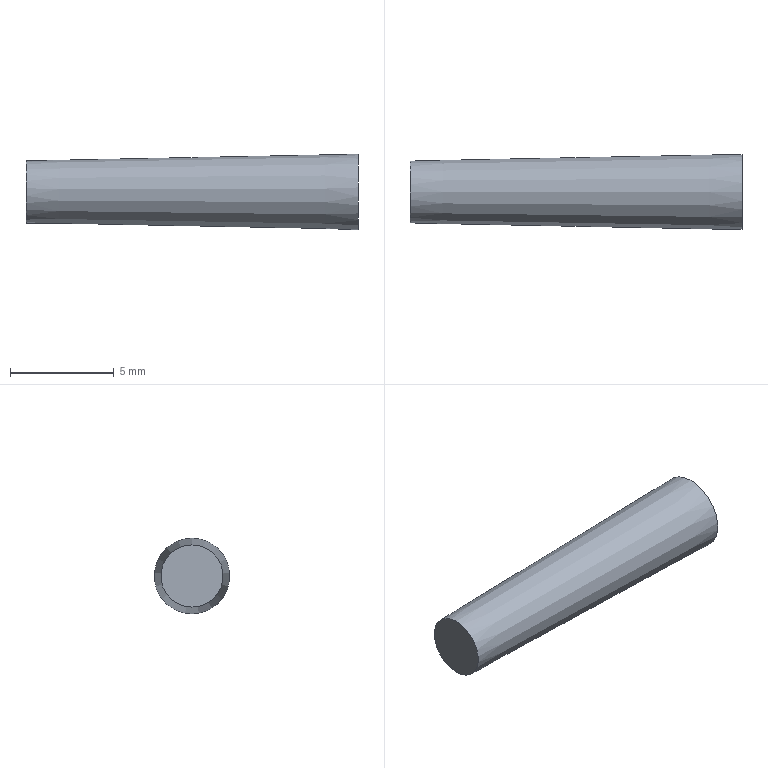Part | NX | features DATUM_CSYS 2, SKETCH 1, SWP104 1 | 1 solid | 3 faces | box 16 x 3.64 x 3.64 mm | volume 138.94 mm3 | plane 2 | cone 1
STEP:
#1=CARTESIAN_POINT('',(16.,0.,1.82));
#2=VERTEX_POINT('',#1);
#3=CARTESIAN_POINT('',(16.,0.,0.));
#4=DIRECTION('',(-1.,0.,0.));
#5=DIRECTION('',(0.,0.,1.));
#6=AXIS2_PLACEMENT_3D('',#3,#4,#5);
#7=CIRCLE('',#6,1.82);
#8=EDGE_CURVE('',#2,#2,#7,.T.);
#9=ORIENTED_EDGE('',*,*,#8,.F.);
#10=EDGE_LOOP('',(#9));
#11=FACE_BOUND('',#10,.T.);
#12=CARTESIAN_POINT('',(16.,0.,0.));
#13=DIRECTION('',(-1.,0.,0.));
#14=DIRECTION('',(0.,0.,1.));
#15=AXIS2_PLACEMENT_3D('',#12,#13,#14);
#16=PLANE('',#15);
#17=ADVANCED_FACE('',(#11),#16,.F.);
#18=CARTESIAN_POINT('',(0.,0.,1.5));
#19=VERTEX_POINT('',#18);
#20=CARTESIAN_POINT('',(0.,0.,0.));
#21=DIRECTION('',(-1.,0.,0.));
#22=DIRECTION('',(0.,0.,1.));
#23=AXIS2_PLACEMENT_3D('',#20,#21,#22);
#24=CIRCLE('',#23,1.5);
#25=EDGE_CURVE('',#19,#19,#24,.T.);
#26=ORIENTED_EDGE('',*,*,#25,.F.);
#27=EDGE_LOOP('',(#26));
#28=FACE_BOUND('',#27,.T.);
#29=ORIENTED_EDGE('',*,*,#8,.T.);
#30=EDGE_LOOP('',(#29));
#31=FACE_BOUND('',#30,.T.);
#32=CARTESIAN_POINT('',(16.,0.,0.));
#33=DIRECTION('',(1.,0.,0.));
#34=DIRECTION('',(0.,0.,-1.));
#35=AXIS2_PLACEMENT_3D('',#32,#33,#34);
#36=CONICAL_SURFACE('',#35,1.82,0.02);
#37=ADVANCED_FACE('',(#28,#31),#36,.T.);
#38=ORIENTED_EDGE('',*,*,#25,.T.);
#39=EDGE_LOOP('',(#38));
#40=FACE_BOUND('',#39,.T.);
#41=CARTESIAN_POINT('',(0.,1.5,0.));
#42=DIRECTION('',(1.,0.,0.));
#43=DIRECTION('',(0.,0.,-1.));
#44=AXIS2_PLACEMENT_3D('',#41,#42,#43);
#45=PLANE('',#44);
#46=ADVANCED_FACE('',(#40),#45,.F.);
#47=CLOSED_SHELL('',(#17,#37,#46));
#48=MANIFOLD_SOLID_BREP('',#47);
#49=(LENGTH_UNIT()NAMED_UNIT(*)SI_UNIT(.MILLI.,.METRE.));
#50=UNCERTAINTY_MEASURE_WITH_UNIT(LENGTH_MEASURE(0.00001),#49,'','');
#51=(NAMED_UNIT(*)PLANE_ANGLE_UNIT()SI_UNIT($,.RADIAN.));
#52=(NAMED_UNIT(*)SI_UNIT($,.STERADIAN.)SOLID_ANGLE_UNIT());
#53=(GEOMETRIC_REPRESENTATION_CONTEXT(3)GLOBAL_UNCERTAINTY_ASSIGNED_CONTEXT((#50))GLOBAL_UNIT_ASSIGNED_CONTEXT((#49,#51,#52))REPRESENTATION_CONTEXT('',''));
#54=ADVANCED_BREP_SHAPE_REPRESENTATION('',(#48),#53);